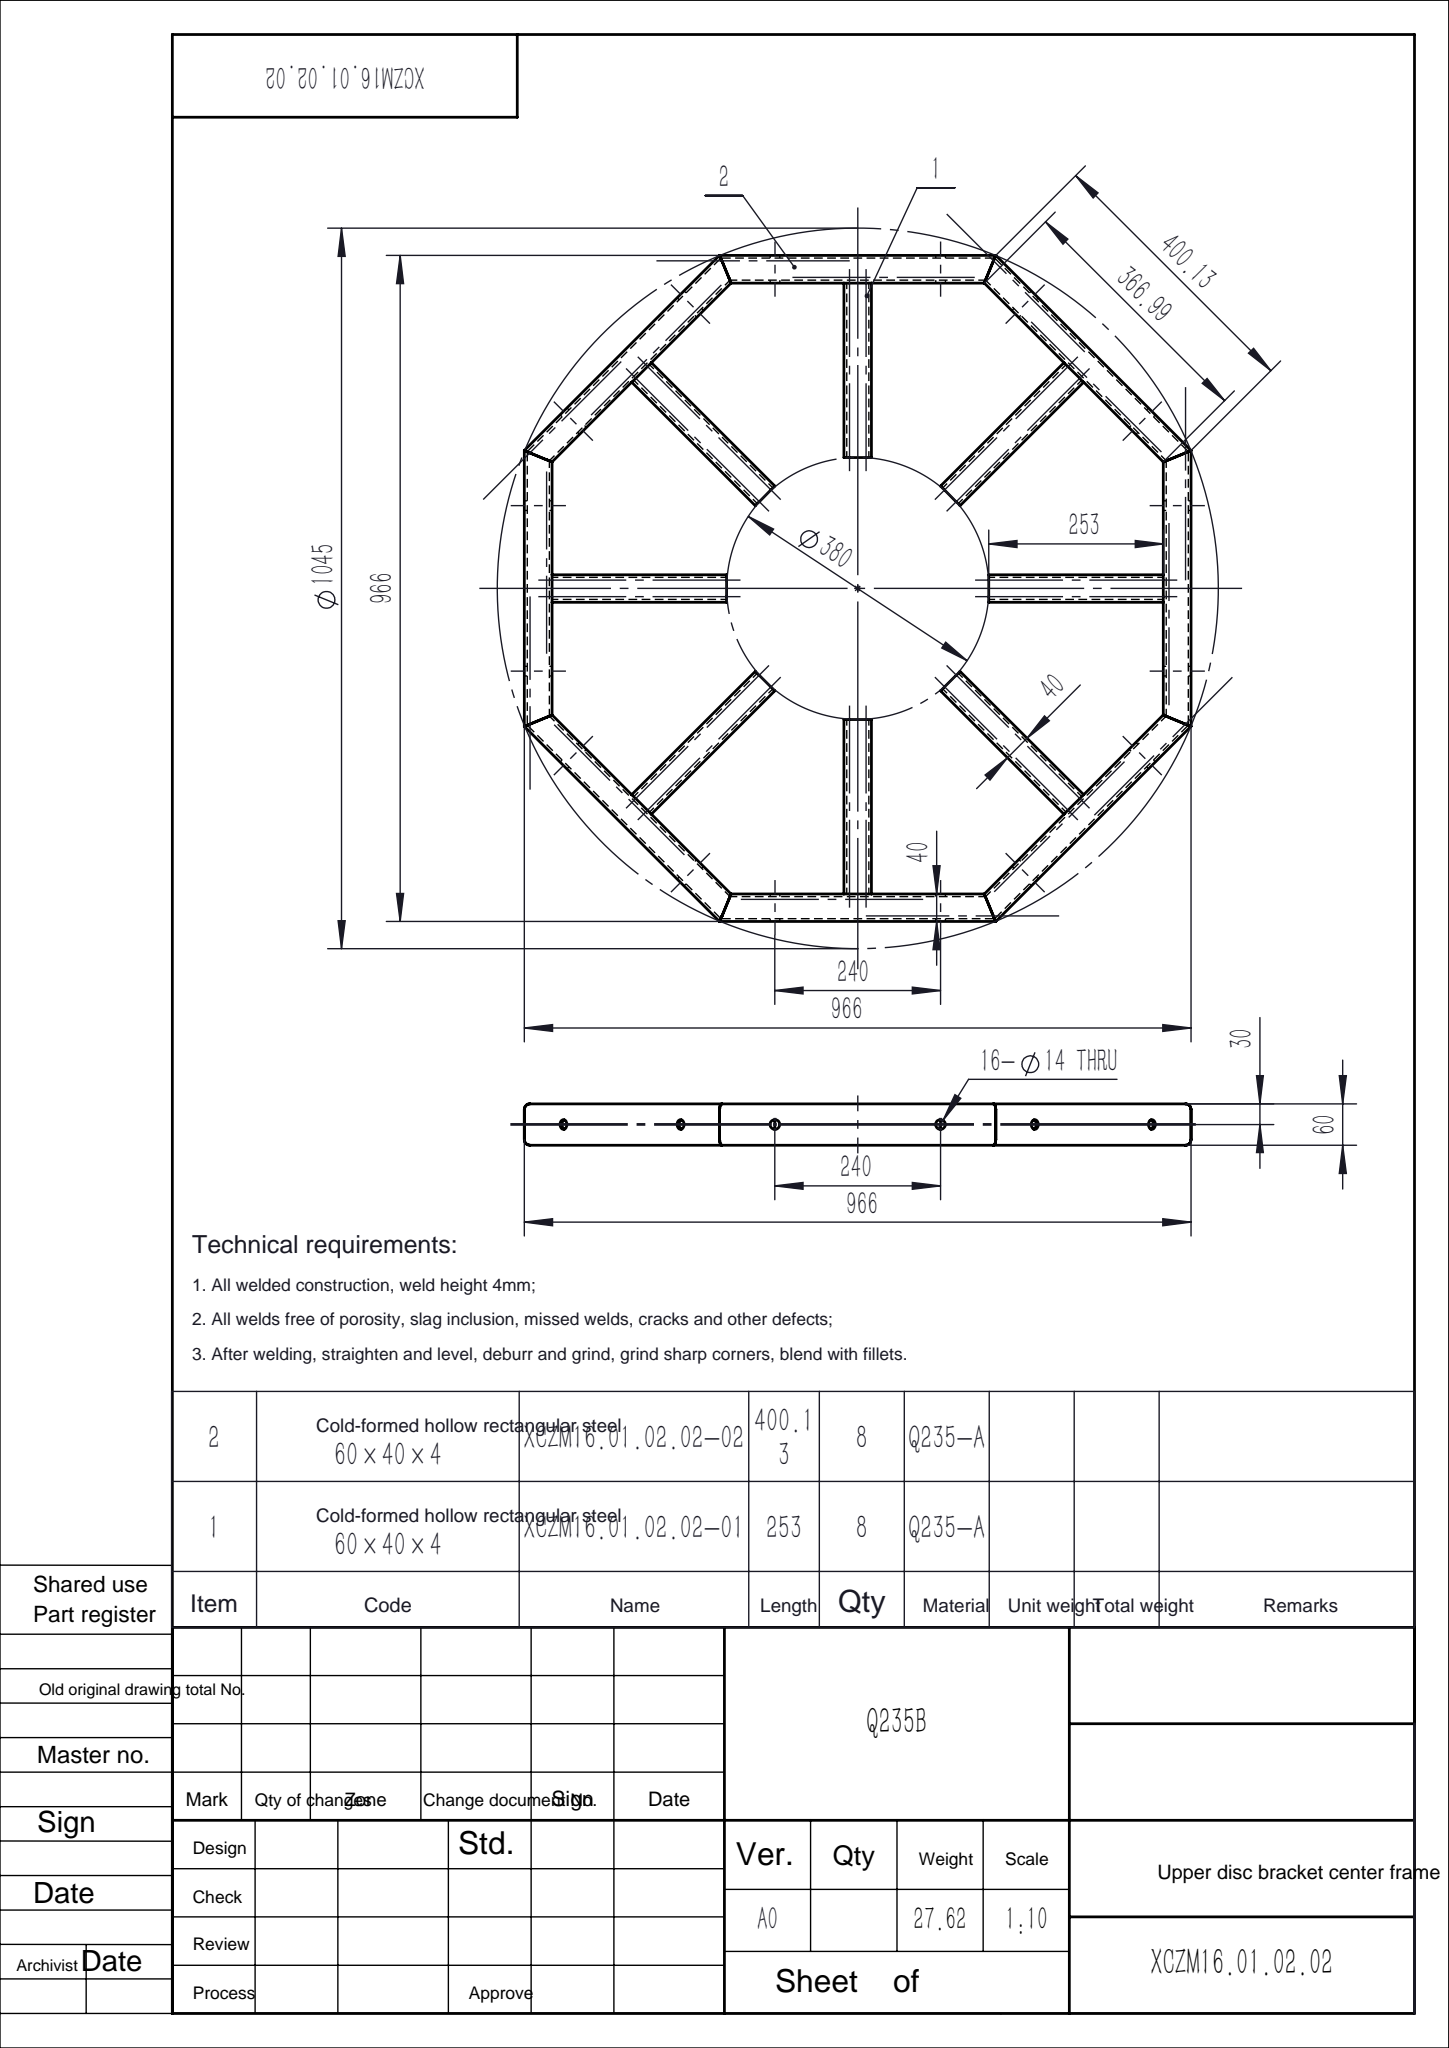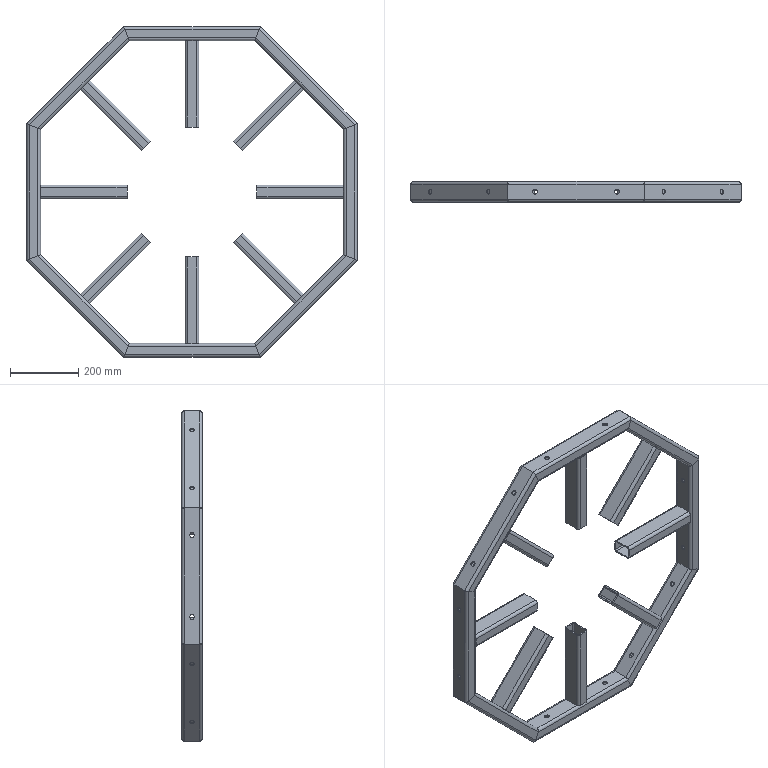Part | SolidWorks | features WeldCornerFeat 8, CirPattern 2, ICE 1, RefAxis 1, WeldMemberFeat 1, WeldmentFeature 1 | 16 solids | 352 faces | box 966 x 60 x 966 mm | volume 3518543 mm3 | cylinder 192 | plane 160 | commonest cylinder face diameters 8 x64 14 x64 16 x64